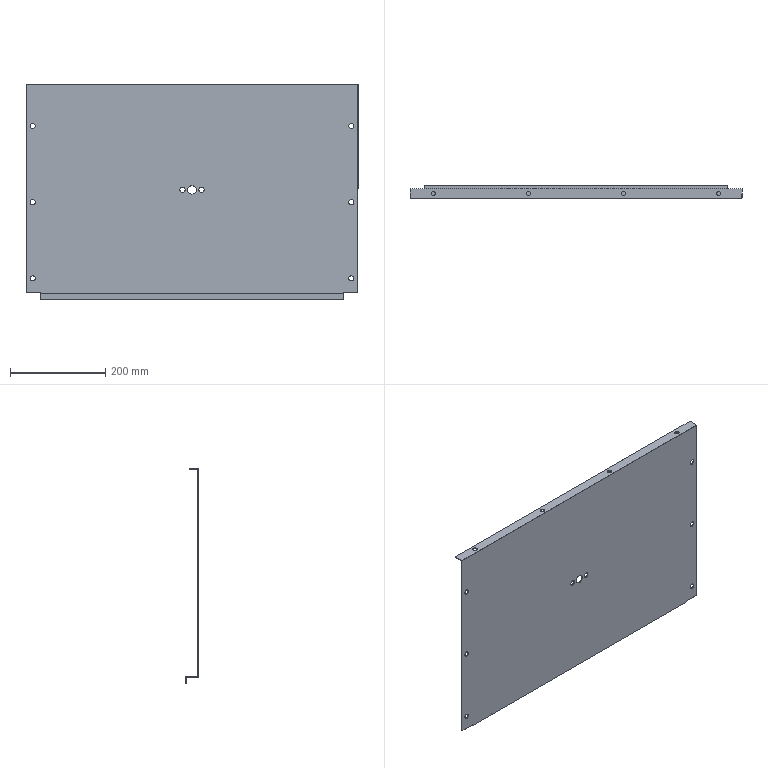Part | SolidWorks | features BaseBody 1 | 1 solid | 42 faces | box 698 x 28 x 453.25 mm | volume 686773 mm3 | cylinder 26 | plane 16 | commonest cylinder face diameters 10.6 x12 9.1 x8 11 x4 18 x2
STEP:
#1=CARTESIAN_POINT('',(211.946,-3643.973,1709.271));
#2=VERTEX_POINT('',#1);
#3=CARTESIAN_POINT('',(211.946,-3643.973,1698.671));
#4=VERTEX_POINT('',#3);
#5=CARTESIAN_POINT('',(211.946,-3643.973,1703.971));
#6=DIRECTION('',(0.,-1.,0.));
#7=DIRECTION('',(0.,0.,-1.));
#8=AXIS2_PLACEMENT_3D('',#5,#6,#7);
#9=CIRCLE('',#8,5.3);
#10=EDGE_CURVE('',#2,#4,#9,.T.);
#11=ORIENTED_EDGE('',*,*,#10,.F.);
#12=CARTESIAN_POINT('',(211.946,-3645.973,1709.271));
#13=VERTEX_POINT('',#12);
#14=CARTESIAN_POINT('',(211.946,-3631.556,1709.271));
#15=DIRECTION('',(0.,-1.,0.));
#16=VECTOR('',#15,1000.);
#17=LINE('',#14,#16);
#18=EDGE_CURVE('',#2,#13,#17,.T.);
#19=ORIENTED_EDGE('',*,*,#18,.T.);
#20=CARTESIAN_POINT('',(211.946,-3645.973,1698.671));
#21=VERTEX_POINT('',#20);
#22=CARTESIAN_POINT('',(211.946,-3645.973,1703.971));
#23=DIRECTION('',(0.,1.,0.));
#24=DIRECTION('',(0.,0.,-1.));
#25=AXIS2_PLACEMENT_3D('',#22,#23,#24);
#26=CIRCLE('',#25,5.3);
#27=EDGE_CURVE('',#21,#13,#26,.T.);
#28=ORIENTED_EDGE('',*,*,#27,.F.);
#29=CARTESIAN_POINT('',(211.946,-3631.556,1698.671));
#30=DIRECTION('',(0.,-1.,0.));
#31=VECTOR('',#30,1000.);
#32=LINE('',#29,#31);
#33=EDGE_CURVE('',#4,#21,#32,.T.);
#34=ORIENTED_EDGE('',*,*,#33,.F.);
#35=EDGE_LOOP('',(#11,#19,#28,#34));
#36=FACE_OUTER_BOUND('',#35,.T.);
#37=CARTESIAN_POINT('',(211.946,-3631.556,1703.971));
#38=DIRECTION('',(0.,-1.,0.));
#39=DIRECTION('',(0.,0.,-1.));
#40=AXIS2_PLACEMENT_3D('',#37,#38,#39);
#41=CYLINDRICAL_SURFACE('',#40,5.3);
#42=ADVANCED_FACE('',(#36),#41,.F.);
#43=CARTESIAN_POINT('',(211.946,-3643.973,2029.271));
#44=VERTEX_POINT('',#43);
#45=CARTESIAN_POINT('',(211.946,-3643.973,2018.671));
#46=VERTEX_POINT('',#45);
#47=CARTESIAN_POINT('',(211.946,-3643.973,2023.971));
#48=DIRECTION('',(0.,-1.,0.));
#49=DIRECTION('',(0.,0.,-1.));
#50=AXIS2_PLACEMENT_3D('',#47,#48,#49);
#51=CIRCLE('',#50,5.3);
#52=EDGE_CURVE('',#44,#46,#51,.T.);
#53=ORIENTED_EDGE('',*,*,#52,.F.);
#54=CARTESIAN_POINT('',(211.946,-3645.973,2029.271));
#55=VERTEX_POINT('',#54);
#56=CARTESIAN_POINT('',(211.946,-3631.556,2029.271));
#57=DIRECTION('',(0.,-1.,0.));
#58=VECTOR('',#57,1000.);
#59=LINE('',#56,#58);
#60=EDGE_CURVE('',#44,#55,#59,.T.);
#61=ORIENTED_EDGE('',*,*,#60,.T.);
#62=CARTESIAN_POINT('',(211.946,-3645.973,2018.671));
#63=VERTEX_POINT('',#62);
#64=CARTESIAN_POINT('',(211.946,-3645.973,2023.971));
#65=DIRECTION('',(0.,1.,0.));
#66=DIRECTION('',(0.,0.,-1.));
#67=AXIS2_PLACEMENT_3D('',#64,#65,#66);
#68=CIRCLE('',#67,5.3);
#69=EDGE_CURVE('',#63,#55,#68,.T.);
#70=ORIENTED_EDGE('',*,*,#69,.F.);
#71=CARTESIAN_POINT('',(211.946,-3631.556,2018.671));
#72=DIRECTION('',(0.,-1.,0.));
#73=VECTOR('',#72,1000.);
#74=LINE('',#71,#73);
#75=EDGE_CURVE('',#46,#63,#74,.T.);
#76=ORIENTED_EDGE('',*,*,#75,.F.);
#77=EDGE_LOOP('',(#53,#61,#70,#76));
#78=FACE_OUTER_BOUND('',#77,.T.);
#79=CARTESIAN_POINT('',(211.946,-3631.556,2023.971));
#80=DIRECTION('',(0.,-1.,0.));
#81=DIRECTION('',(0.,0.,-1.));
#82=AXIS2_PLACEMENT_3D('',#79,#80,#81);
#83=CYLINDRICAL_SURFACE('',#82,5.3);
#84=ADVANCED_FACE('',(#78),#83,.F.);
#85=CARTESIAN_POINT('',(881.946,-3645.973,1858.671));
#86=VERTEX_POINT('',#85);
#87=CARTESIAN_POINT('',(881.946,-3645.973,1869.271));
#88=VERTEX_POINT('',#87);
#89=CARTESIAN_POINT('',(881.946,-3645.973,1863.971));
#90=DIRECTION('',(0.,1.,0.));
#91=DIRECTION('',(0.,0.,1.));
#92=AXIS2_PLACEMENT_3D('',#89,#90,#91);
#93=CIRCLE('',#92,5.3);
#94=EDGE_CURVE('',#86,#88,#93,.T.);
#95=ORIENTED_EDGE('',*,*,#94,.F.);
#96=CARTESIAN_POINT('',(881.946,-3643.973,1858.671));
#97=VERTEX_POINT('',#96);
#98=CARTESIAN_POINT('',(881.946,-3631.556,1858.671));
#99=DIRECTION('',(0.,1.,0.));
#100=VECTOR('',#99,1000.);
#101=LINE('',#98,#100);
#102=EDGE_CURVE('',#86,#97,#101,.T.);
#103=ORIENTED_EDGE('',*,*,#102,.T.);
#104=CARTESIAN_POINT('',(881.946,-3643.973,1869.271));
#105=VERTEX_POINT('',#104);
#106=CARTESIAN_POINT('',(881.946,-3643.973,1863.971));
#107=DIRECTION('',(0.,-1.,0.));
#108=DIRECTION('',(0.,0.,1.));
#109=AXIS2_PLACEMENT_3D('',#106,#107,#108);
#110=CIRCLE('',#109,5.3);
#111=EDGE_CURVE('',#105,#97,#110,.T.);
#112=ORIENTED_EDGE('',*,*,#111,.F.);
#113=CARTESIAN_POINT('',(881.946,-3631.556,1869.271));
#114=DIRECTION('',(0.,1.,0.));
#115=VECTOR('',#114,1000.);
#116=LINE('',#113,#115);
#117=EDGE_CURVE('',#88,#105,#116,.T.);
#118=ORIENTED_EDGE('',*,*,#117,.F.);
#119=EDGE_LOOP('',(#95,#103,#112,#118));
#120=FACE_OUTER_BOUND('',#119,.T.);
#121=CARTESIAN_POINT('',(881.946,-3631.556,1863.971));
#122=DIRECTION('',(0.,1.,0.));
#123=DIRECTION('',(0.,0.,1.));
#124=AXIS2_PLACEMENT_3D('',#121,#122,#123);
#125=CYLINDRICAL_SURFACE('',#124,5.3);
#126=ADVANCED_FACE('',(#120),#125,.F.);
#127=CARTESIAN_POINT('',(881.946,-3645.973,2018.671));
#128=VERTEX_POINT('',#127);
#129=CARTESIAN_POINT('',(881.946,-3645.973,2029.271));
#130=VERTEX_POINT('',#129);
#131=CARTESIAN_POINT('',(881.946,-3645.973,2023.971));
#132=DIRECTION('',(0.,1.,0.));
#133=DIRECTION('',(0.,0.,1.));
#134=AXIS2_PLACEMENT_3D('',#131,#132,#133);
#135=CIRCLE('',#134,5.3);
#136=EDGE_CURVE('',#128,#130,#135,.T.);
#137=ORIENTED_EDGE('',*,*,#136,.F.);
#138=CARTESIAN_POINT('',(881.946,-3643.973,2018.671));
#139=VERTEX_POINT('',#138);
#140=CARTESIAN_POINT('',(881.946,-3631.556,2018.671));
#141=DIRECTION('',(0.,1.,0.));
#142=VECTOR('',#141,1000.);
#143=LINE('',#140,#142);
#144=EDGE_CURVE('',#128,#139,#143,.T.);
#145=ORIENTED_EDGE('',*,*,#144,.T.);
#146=CARTESIAN_POINT('',(881.946,-3643.973,2029.271));
#147=VERTEX_POINT('',#146);
#148=CARTESIAN_POINT('',(881.946,-3643.973,2023.971));
#149=DIRECTION('',(0.,-1.,0.));
#150=DIRECTION('',(0.,0.,1.));
#151=AXIS2_PLACEMENT_3D('',#148,#149,#150);
#152=CIRCLE('',#151,5.3);
#153=EDGE_CURVE('',#147,#139,#152,.T.);
#154=ORIENTED_EDGE('',*,*,#153,.F.);
#155=CARTESIAN_POINT('',(881.946,-3631.556,2029.271));
#156=DIRECTION('',(0.,1.,0.));
#157=VECTOR('',#156,1000.);
#158=LINE('',#155,#157);
#159=EDGE_CURVE('',#130,#147,#158,.T.);
#160=ORIENTED_EDGE('',*,*,#159,.F.);
#161=EDGE_LOOP('',(#137,#145,#154,#160));
#162=FACE_OUTER_BOUND('',#161,.T.);
#163=CARTESIAN_POINT('',(881.946,-3631.556,2023.971));
#164=DIRECTION('',(0.,1.,0.));
#165=DIRECTION('',(0.,0.,1.));
#166=AXIS2_PLACEMENT_3D('',#163,#164,#165);
#167=CYLINDRICAL_SURFACE('',#166,5.3);
#168=ADVANCED_FACE('',(#162),#167,.F.);
#169=CARTESIAN_POINT('',(881.946,-3645.973,1698.671));
#170=VERTEX_POINT('',#169);
#171=CARTESIAN_POINT('',(881.946,-3645.973,1709.271));
#172=VERTEX_POINT('',#171);
#173=CARTESIAN_POINT('',(881.946,-3645.973,1703.971));
#174=DIRECTION('',(0.,1.,0.));
#175=DIRECTION('',(0.,0.,1.));
#176=AXIS2_PLACEMENT_3D('',#173,#174,#175);
#177=CIRCLE('',#176,5.3);
#178=EDGE_CURVE('',#170,#172,#177,.T.);
#179=ORIENTED_EDGE('',*,*,#178,.F.);
#180=CARTESIAN_POINT('',(881.946,-3643.973,1698.671));
#181=VERTEX_POINT('',#180);
#182=CARTESIAN_POINT('',(881.946,-3631.556,1698.671));
#183=DIRECTION('',(0.,1.,0.));
#184=VECTOR('',#183,1000.);
#185=LINE('',#182,#184);
#186=EDGE_CURVE('',#170,#181,#185,.T.);
#187=ORIENTED_EDGE('',*,*,#186,.T.);
#188=CARTESIAN_POINT('',(881.946,-3643.973,1709.271));
#189=VERTEX_POINT('',#188);
#190=CARTESIAN_POINT('',(881.946,-3643.973,1703.971));
#191=DIRECTION('',(0.,-1.,0.));
#192=DIRECTION('',(0.,0.,1.));
#193=AXIS2_PLACEMENT_3D('',#190,#191,#192);
#194=CIRCLE('',#193,5.3);
#195=EDGE_CURVE('',#189,#181,#194,.T.);
#196=ORIENTED_EDGE('',*,*,#195,.F.);
#197=CARTESIAN_POINT('',(881.946,-3631.556,1709.271));
#198=DIRECTION('',(0.,1.,0.));
#199=VECTOR('',#198,1000.);
#200=LINE('',#197,#199);
#201=EDGE_CURVE('',#172,#189,#200,.T.);
#202=ORIENTED_EDGE('',*,*,#201,.F.);
#203=EDGE_LOOP('',(#179,#187,#196,#202));
#204=FACE_OUTER_BOUND('',#203,.T.);
#205=CARTESIAN_POINT('',(881.946,-3631.556,1703.971));
#206=DIRECTION('',(0.,1.,0.));
#207=DIRECTION('',(0.,0.,1.));
#208=AXIS2_PLACEMENT_3D('',#205,#206,#207);
#209=CYLINDRICAL_SURFACE('',#208,5.3);
#210=ADVANCED_FACE('',(#204),#209,.F.);
#211=CARTESIAN_POINT('',(211.946,-3643.973,1869.271));
#212=VERTEX_POINT('',#211);
#213=CARTESIAN_POINT('',(211.946,-3643.973,1858.671));
#214=VERTEX_POINT('',#213);
#215=CARTESIAN_POINT('',(211.946,-3643.973,1863.971));
#216=DIRECTION('',(0.,-1.,0.));
#217=DIRECTION('',(0.,0.,-1.));
#218=AXIS2_PLACEMENT_3D('',#215,#216,#217);
#219=CIRCLE('',#218,5.3);
#220=EDGE_CURVE('',#212,#214,#219,.T.);
#221=ORIENTED_EDGE('',*,*,#220,.F.);
#222=CARTESIAN_POINT('',(211.946,-3645.973,1869.271));
#223=VERTEX_POINT('',#222);
#224=CARTESIAN_POINT('',(211.946,-3631.556,1869.271));
#225=DIRECTION('',(0.,-1.,0.));
#226=VECTOR('',#225,1000.);
#227=LINE('',#224,#226);
#228=EDGE_CURVE('',#212,#223,#227,.T.);
#229=ORIENTED_EDGE('',*,*,#228,.T.);
#230=CARTESIAN_POINT('',(211.946,-3645.973,1858.671));
#231=VERTEX_POINT('',#230);
#232=CARTESIAN_POINT('',(211.946,-3645.973,1863.971));
#233=DIRECTION('',(0.,1.,0.));
#234=DIRECTION('',(0.,0.,-1.));
#235=AXIS2_PLACEMENT_3D('',#232,#233,#234);
#236=CIRCLE('',#235,5.3);
#237=EDGE_CURVE('',#231,#223,#236,.T.);
#238=ORIENTED_EDGE('',*,*,#237,.F.);
#239=CARTESIAN_POINT('',(211.946,-3631.556,1858.671));
#240=DIRECTION('',(0.,-1.,0.));
#241=VECTOR('',#240,1000.);
#242=LINE('',#239,#241);
#243=EDGE_CURVE('',#214,#231,#242,.T.);
#244=ORIENTED_EDGE('',*,*,#243,.F.);
#245=EDGE_LOOP('',(#221,#229,#238,#244));
#246=FACE_OUTER_BOUND('',#245,.T.);
#247=CARTESIAN_POINT('',(211.946,-3631.556,1863.971));
#248=DIRECTION('',(0.,-1.,0.));
#249=DIRECTION('',(0.,0.,-1.));
#250=AXIS2_PLACEMENT_3D('',#247,#248,#249);
#251=CYLINDRICAL_SURFACE('',#250,5.3);
#252=ADVANCED_FACE('',(#246),#251,.F.);
#253=CARTESIAN_POINT('',(526.946,-3643.973,1895.471));
#254=VERTEX_POINT('',#253);
#255=CARTESIAN_POINT('',(526.946,-3643.973,1884.471));
#256=VERTEX_POINT('',#255);
#257=CARTESIAN_POINT('',(526.946,-3643.973,1889.971));
#258=DIRECTION('',(0.,-1.,0.));
#259=DIRECTION('',(0.,0.,-1.));
#260=AXIS2_PLACEMENT_3D('',#257,#258,#259);
#261=CIRCLE('',#260,5.5);
#262=EDGE_CURVE('',#254,#256,#261,.T.);
#263=ORIENTED_EDGE('',*,*,#262,.F.);
#264=CARTESIAN_POINT('',(526.946,-3645.973,1895.471));
#265=VERTEX_POINT('',#264);
#266=CARTESIAN_POINT('',(526.946,-3653.934,1895.471));
#267=DIRECTION('',(0.,-1.,0.));
#268=VECTOR('',#267,1000.);
#269=LINE('',#266,#268);
#270=EDGE_CURVE('',#254,#265,#269,.T.);
#271=ORIENTED_EDGE('',*,*,#270,.T.);
#272=CARTESIAN_POINT('',(526.946,-3645.973,1884.471));
#273=VERTEX_POINT('',#272);
#274=CARTESIAN_POINT('',(526.946,-3645.973,1889.971));
#275=DIRECTION('',(0.,1.,0.));
#276=DIRECTION('',(0.,0.,-1.));
#277=AXIS2_PLACEMENT_3D('',#274,#275,#276);
#278=CIRCLE('',#277,5.5);
#279=EDGE_CURVE('',#273,#265,#278,.T.);
#280=ORIENTED_EDGE('',*,*,#279,.F.);
#281=CARTESIAN_POINT('',(526.946,-3653.934,1884.471));
#282=DIRECTION('',(0.,-1.,0.));
#283=VECTOR('',#282,1000.);
#284=LINE('',#281,#283);
#285=EDGE_CURVE('',#256,#273,#284,.T.);
#286=ORIENTED_EDGE('',*,*,#285,.F.);
#287=EDGE_LOOP('',(#263,#271,#280,#286));
#288=FACE_OUTER_BOUND('',#287,.T.);
#289=CARTESIAN_POINT('',(526.946,-3653.934,1889.971));
#290=DIRECTION('',(0.,-1.,0.));
#291=DIRECTION('',(0.,0.,-1.));
#292=AXIS2_PLACEMENT_3D('',#289,#290,#291);
#293=CYLINDRICAL_SURFACE('',#292,5.5);
#294=ADVANCED_FACE('',(#288),#293,.F.);
#295=CARTESIAN_POINT('',(566.946,-3645.973,1884.471));
#296=VERTEX_POINT('',#295);
#297=CARTESIAN_POINT('',(566.946,-3645.973,1895.471));
#298=VERTEX_POINT('',#297);
#299=CARTESIAN_POINT('',(566.946,-3645.973,1889.971));
#300=DIRECTION('',(0.,1.,0.));
#301=DIRECTION('',(0.,0.,1.));
#302=AXIS2_PLACEMENT_3D('',#299,#300,#301);
#303=CIRCLE('',#302,5.5);
#304=EDGE_CURVE('',#296,#298,#303,.T.);
#305=ORIENTED_EDGE('',*,*,#304,.F.);
#306=CARTESIAN_POINT('',(566.946,-3643.973,1884.471));
#307=VERTEX_POINT('',#306);
#308=CARTESIAN_POINT('',(566.946,-3653.934,1884.471));
#309=DIRECTION('',(0.,1.,0.));
#310=VECTOR('',#309,1000.);
#311=LINE('',#308,#310);
#312=EDGE_CURVE('',#296,#307,#311,.T.);
#313=ORIENTED_EDGE('',*,*,#312,.T.);
#314=CARTESIAN_POINT('',(566.946,-3643.973,1895.471));
#315=VERTEX_POINT('',#314);
#316=CARTESIAN_POINT('',(566.946,-3643.973,1889.971));
#317=DIRECTION('',(0.,-1.,0.));
#318=DIRECTION('',(0.,0.,1.));
#319=AXIS2_PLACEMENT_3D('',#316,#317,#318);
#320=CIRCLE('',#319,5.5);
#321=EDGE_CURVE('',#315,#307,#320,.T.);
#322=ORIENTED_EDGE('',*,*,#321,.F.);
#323=CARTESIAN_POINT('',(566.946,-3653.934,1895.471));
#324=DIRECTION('',(0.,1.,0.));
#325=VECTOR('',#324,1000.);
#326=LINE('',#323,#325);
#327=EDGE_CURVE('',#298,#315,#326,.T.);
#328=ORIENTED_EDGE('',*,*,#327,.F.);
#329=EDGE_LOOP('',(#305,#313,#322,#328));
#330=FACE_OUTER_BOUND('',#329,.T.);
#331=CARTESIAN_POINT('',(566.946,-3653.934,1889.971));
#332=DIRECTION('',(0.,1.,0.));
#333=DIRECTION('',(0.,0.,1.));
#334=AXIS2_PLACEMENT_3D('',#331,#332,#333);
#335=CYLINDRICAL_SURFACE('',#334,5.5);
#336=ADVANCED_FACE('',(#330),#335,.F.);
#337=CARTESIAN_POINT('',(546.946,-3643.973,1898.971));
#338=VERTEX_POINT('',#337);
#339=CARTESIAN_POINT('',(546.946,-3643.973,1880.971));
#340=VERTEX_POINT('',#339);
#341=CARTESIAN_POINT('',(546.946,-3643.973,1889.971));
#342=DIRECTION('',(0.,-1.,0.));
#343=DIRECTION('',(0.,0.,-1.));
#344=AXIS2_PLACEMENT_3D('',#341,#342,#343);
#345=CIRCLE('',#344,9.);
#346=EDGE_CURVE('',#338,#340,#345,.T.);
#347=ORIENTED_EDGE('',*,*,#346,.F.);
#348=CARTESIAN_POINT('',(546.946,-3645.973,1898.971));
#349=VERTEX_POINT('',#348);
#350=CARTESIAN_POINT('',(546.946,-3642.444,1898.971));
#351=DIRECTION('',(0.,-1.,0.));
#352=VECTOR('',#351,1000.);
#353=LINE('',#350,#352);
#354=EDGE_CURVE('',#338,#349,#353,.T.);
#355=ORIENTED_EDGE('',*,*,#354,.T.);
#356=CARTESIAN_POINT('',(546.946,-3645.973,1880.971));
#357=VERTEX_POINT('',#356);
#358=CARTESIAN_POINT('',(546.946,-3645.973,1889.971));
#359=DIRECTION('',(0.,1.,0.));
#360=DIRECTION('',(0.,0.,-1.));
#361=AXIS2_PLACEMENT_3D('',#358,#359,#360);
#362=CIRCLE('',#361,9.);
#363=EDGE_CURVE('',#357,#349,#362,.T.);
#364=ORIENTED_EDGE('',*,*,#363,.F.);
#365=CARTESIAN_POINT('',(546.946,-3642.444,1880.971));
#366=DIRECTION('',(0.,-1.,0.));
#367=VECTOR('',#366,1000.);
#368=LINE('',#365,#367);
#369=EDGE_CURVE('',#340,#357,#368,.T.);
#370=ORIENTED_EDGE('',*,*,#369,.F.);
#371=EDGE_LOOP('',(#347,#355,#364,#370));
#372=FACE_OUTER_BOUND('',#371,.T.);
#373=CARTESIAN_POINT('',(546.946,-3642.444,1889.971));
#374=DIRECTION('',(0.,-1.,0.));
#375=DIRECTION('',(0.,0.,-1.));
#376=AXIS2_PLACEMENT_3D('',#373,#374,#375);
#377=CYLINDRICAL_SURFACE('',#376,9.);
#378=ADVANCED_FACE('',(#372),#377,.F.);
#379=CARTESIAN_POINT('',(242.396,-3635.973,2109.971));
#380=VERTEX_POINT('',#379);
#381=CARTESIAN_POINT('',(251.496,-3635.973,2109.971));
#382=VERTEX_POINT('',#381);
#383=CARTESIAN_POINT('',(246.946,-3635.973,2109.971));
#384=DIRECTION('',(0.,0.,1.));
#385=DIRECTION('',(1.,0.,0.));
#386=AXIS2_PLACEMENT_3D('',#383,#384,#385);
#387=CIRCLE('',#386,4.55);
#388=EDGE_CURVE('',#380,#382,#387,.T.);
#389=ORIENTED_EDGE('',*,*,#388,.F.);
#390=CARTESIAN_POINT('',(242.396,-3635.973,2111.971));
#391=VERTEX_POINT('',#390);
#392=CARTESIAN_POINT('',(242.396,-3635.973,2133.845));
#393=DIRECTION('',(0.,0.,1.));
#394=VECTOR('',#393,1000.);
#395=LINE('',#392,#394);
#396=EDGE_CURVE('',#380,#391,#395,.T.);
#397=ORIENTED_EDGE('',*,*,#396,.T.);
#398=CARTESIAN_POINT('',(251.496,-3635.973,2111.971));
#399=VERTEX_POINT('',#398);
#400=CARTESIAN_POINT('',(246.946,-3635.973,2111.971));
#401=DIRECTION('',(0.,0.,-1.));
#402=DIRECTION('',(1.,0.,0.));
#403=AXIS2_PLACEMENT_3D('',#400,#401,#402);
#404=CIRCLE('',#403,4.55);
#405=EDGE_CURVE('',#399,#391,#404,.T.);
#406=ORIENTED_EDGE('',*,*,#405,.F.);
#407=CARTESIAN_POINT('',(251.496,-3635.973,2133.845));
#408=DIRECTION('',(0.,0.,1.));
#409=VECTOR('',#408,1000.);
#410=LINE('',#407,#409);
#411=EDGE_CURVE('',#382,#399,#410,.T.);
#412=ORIENTED_EDGE('',*,*,#411,.F.);
#413=EDGE_LOOP('',(#389,#397,#406,#412));
#414=FACE_OUTER_BOUND('',#413,.T.);
#415=CARTESIAN_POINT('',(246.946,-3635.973,2133.845));
#416=DIRECTION('',(0.,0.,1.));
#417=DIRECTION('',(1.,0.,0.));
#418=AXIS2_PLACEMENT_3D('',#415,#416,#417);
#419=CYLINDRICAL_SURFACE('',#418,4.55);
#420=ADVANCED_FACE('',(#414),#419,.F.);
#421=CARTESIAN_POINT('',(851.496,-3635.973,2111.971));
#422=VERTEX_POINT('',#421);
#423=CARTESIAN_POINT('',(842.396,-3635.973,2111.971));
#424=VERTEX_POINT('',#423);
#425=CARTESIAN_POINT('',(846.946,-3635.973,2111.971));
#426=DIRECTION('',(0.,0.,-1.));
#427=DIRECTION('',(-1.,0.,0.));
#428=AXIS2_PLACEMENT_3D('',#425,#426,#427);
#429=CIRCLE('',#428,4.55);
#430=EDGE_CURVE('',#422,#424,#429,.T.);
#431=ORIENTED_EDGE('',*,*,#430,.F.);
#432=CARTESIAN_POINT('',(851.496,-3635.973,2109.971));
#433=VERTEX_POINT('',#432);
#434=CARTESIAN_POINT('',(851.496,-3635.973,2133.845));
#435=DIRECTION('',(0.,0.,-1.));
#436=VECTOR('',#435,1000.);
#437=LINE('',#434,#436);
#438=EDGE_CURVE('',#422,#433,#437,.T.);
#439=ORIENTED_EDGE('',*,*,#438,.T.);
#440=CARTESIAN_POINT('',(842.396,-3635.973,2109.971));
#441=VERTEX_POINT('',#440);
#442=CARTESIAN_POINT('',(846.946,-3635.973,2109.971));
#443=DIRECTION('',(0.,0.,1.));
#444=DIRECTION('',(-1.,0.,0.));
#445=AXIS2_PLACEMENT_3D('',#442,#443,#444);
#446=CIRCLE('',#445,4.55);
#447=EDGE_CURVE('',#441,#433,#446,.T.);
#448=ORIENTED_EDGE('',*,*,#447,.F.);
#449=CARTESIAN_POINT('',(842.396,-3635.973,2133.845));
#450=DIRECTION('',(0.,0.,-1.));
#451=VECTOR('',#450,1000.);
#452=LINE('',#449,#451);
#453=EDGE_CURVE('',#424,#441,#452,.T.);
#454=ORIENTED_EDGE('',*,*,#453,.F.);
#455=EDGE_LOOP('',(#431,#439,#448,#454));
#456=FACE_OUTER_BOUND('',#455,.T.);
#457=CARTESIAN_POINT('',(846.946,-3635.973,2133.845));
#458=DIRECTION('',(0.,0.,-1.));
#459=DIRECTION('',(-1.,0.,0.));
#460=AXIS2_PLACEMENT_3D('',#457,#458,#459);
#461=CYLINDRICAL_SURFACE('',#460,4.55);
#462=ADVANCED_FACE('',(#456),#461,.F.);
#463=CARTESIAN_POINT('',(651.496,-3635.973,2111.971));
#464=VERTEX_POINT('',#463);
#465=CARTESIAN_POINT('',(642.396,-3635.973,2111.971));
#466=VERTEX_POINT('',#465);
#467=CARTESIAN_POINT('',(646.946,-3635.973,2111.971));
#468=DIRECTION('',(0.,0.,-1.));
#469=DIRECTION('',(-1.,0.,0.));
#470=AXIS2_PLACEMENT_3D('',#467,#468,#469);
#471=CIRCLE('',#470,4.55);
#472=EDGE_CURVE('',#464,#466,#471,.T.);
#473=ORIENTED_EDGE('',*,*,#472,.F.);
#474=CARTESIAN_POINT('',(651.496,-3635.973,2109.971));
#475=VERTEX_POINT('',#474);
#476=CARTESIAN_POINT('',(651.496,-3635.973,2133.845));
#477=DIRECTION('',(0.,0.,-1.));
#478=VECTOR('',#477,1000.);
#479=LINE('',#476,#478);
#480=EDGE_CURVE('',#464,#475,#479,.T.);
#481=ORIENTED_EDGE('',*,*,#480,.T.);
#482=CARTESIAN_POINT('',(642.396,-3635.973,2109.971));
#483=VERTEX_POINT('',#482);
#484=CARTESIAN_POINT('',(646.946,-3635.973,2109.971));
#485=DIRECTION('',(0.,0.,1.));
#486=DIRECTION('',(-1.,0.,0.));
#487=AXIS2_PLACEMENT_3D('',#484,#485,#486);
#488=CIRCLE('',#487,4.55);
#489=EDGE_CURVE('',#483,#475,#488,.T.);
#490=ORIENTED_EDGE('',*,*,#489,.F.);
#491=CARTESIAN_POINT('',(642.396,-3635.973,2133.845));
#492=DIRECTION('',(0.,0.,-1.));
#493=VECTOR('',#492,1000.);
#494=LINE('',#491,#493);
#495=EDGE_CURVE('',#466,#483,#494,.T.);
#496=ORIENTED_EDGE('',*,*,#495,.F.);
#497=EDGE_LOOP('',(#473,#481,#490,#496));
#498=FACE_OUTER_BOUND('',#497,.T.);
#499=CARTESIAN_POINT('',(646.946,-3635.973,2133.845));
#500=DIRECTION('',(0.,0.,-1.));
#501=DIRECTION('',(-1.,0.,0.));
#502=AXIS2_PLACEMENT_3D('',#499,#500,#501);
#503=CYLINDRICAL_SURFACE('',#502,4.55);
#504=ADVANCED_FACE('',(#498),#503,.F.);
#505=CARTESIAN_POINT('',(442.396,-3635.973,2109.971));
#506=VERTEX_POINT('',#505);
#507=CARTESIAN_POINT('',(451.496,-3635.973,2109.971));
#508=VERTEX_POINT('',#507);
#509=CARTESIAN_POINT('',(446.946,-3635.973,2109.971));
#510=DIRECTION('',(0.,0.,1.));
#511=DIRECTION('',(1.,0.,0.));
#512=AXIS2_PLACEMENT_3D('',#509,#510,#511);
#513=CIRCLE('',#512,4.55);
#514=EDGE_CURVE('',#506,#508,#513,.T.);
#515=ORIENTED_EDGE('',*,*,#514,.F.);
#516=CARTESIAN_POINT('',(442.396,-3635.973,2111.971));
#517=VERTEX_POINT('',#516);
#518=CARTESIAN_POINT('',(442.396,-3635.973,2133.845));
#519=DIRECTION('',(0.,0.,1.));
#520=VECTOR('',#519,1000.);
#521=LINE('',#518,#520);
#522=EDGE_CURVE('',#506,#517,#521,.T.);
#523=ORIENTED_EDGE('',*,*,#522,.T.);
#524=CARTESIAN_POINT('',(451.496,-3635.973,2111.971));
#525=VERTEX_POINT('',#524);
#526=CARTESIAN_POINT('',(446.946,-3635.973,2111.971));
#527=DIRECTION('',(0.,0.,-1.));
#528=DIRECTION('',(1.,0.,0.));
#529=AXIS2_PLACEMENT_3D('',#526,#527,#528);
#530=CIRCLE('',#529,4.55);
#531=EDGE_CURVE('',#525,#517,#530,.T.);
#532=ORIENTED_EDGE('',*,*,#531,.F.);
#533=CARTESIAN_POINT('',(451.496,-3635.973,2133.845));
#534=DIRECTION('',(0.,0.,1.));
#535=VECTOR('',#534,1000.);
#536=LINE('',#533,#535);
#537=EDGE_CURVE('',#508,#525,#536,.T.);
#538=ORIENTED_EDGE('',*,*,#537,.F.);
#539=EDGE_LOOP('',(#515,#523,#532,#538));
#540=FACE_OUTER_BOUND('',#539,.T.);
#541=CARTESIAN_POINT('',(446.946,-3635.973,2133.845));
#542=DIRECTION('',(0.,0.,1.));
#543=DIRECTION('',(1.,0.,0.));
#544=AXIS2_PLACEMENT_3D('',#541,#542,#543);
#545=CYLINDRICAL_SURFACE('',#544,4.55);
#546=ADVANCED_FACE('',(#540),#545,.F.);
#547=CARTESIAN_POINT('',(895.946,-3645.973,1673.721));
#548=VERTEX_POINT('',#547);
#549=CARTESIAN_POINT('',(895.946,-3645.973,2111.971));
#550=VERTEX_POINT('',#549);
#551=CARTESIAN_POINT('',(895.946,-3645.973,2111.971));
#552=DIRECTION('',(0.,0.,1.));
#553=VECTOR('',#552,1000.);
#554=LINE('',#551,#553);
#555=EDGE_CURVE('',#548,#550,#554,.T.);
#556=ORIENTED_EDGE('',*,*,#555,.T.);
#557=CARTESIAN_POINT('',(197.946,-3645.973,2111.971));
#558=VERTEX_POINT('',#557);
#559=CARTESIAN_POINT('',(895.946,-3645.973,2111.971));
#560=DIRECTION('',(-1.,0.,0.));
#561=VECTOR('',#560,1000.);
#562=LINE('',#559,#561);
#563=EDGE_CURVE('',#550,#558,#562,.T.);
#564=ORIENTED_EDGE('',*,*,#563,.T.);
#565=CARTESIAN_POINT('',(197.946,-3645.973,1673.721));
#566=VERTEX_POINT('',#565);
#567=CARTESIAN_POINT('',(197.946,-3645.973,2111.971));
#568=DIRECTION('',(0.,0.,-1.));
#569=VECTOR('',#568,1000.);
#570=LINE('',#567,#569);
#571=EDGE_CURVE('',#558,#566,#570,.T.);
#572=ORIENTED_EDGE('',*,*,#571,.T.);
#573=CARTESIAN_POINT('',(227.946,-3645.973,1673.721));
#574=VERTEX_POINT('',#573);
#575=CARTESIAN_POINT('',(895.946,-3645.973,1673.721));
#576=DIRECTION('',(1.,0.,0.));
#577=VECTOR('',#576,1000.);
#578=LINE('',#575,#577);
#579=EDGE_CURVE('',#566,#574,#578,.T.);
#580=ORIENTED_EDGE('',*,*,#579,.T.);
#581=CARTESIAN_POINT('',(227.946,-3645.973,1671.721));
#582=VERTEX_POINT('',#581);
#583=CARTESIAN_POINT('',(227.946,-3645.973,2111.971));
#584=DIRECTION('',(0.,0.,-1.));
#585=VECTOR('',#584,1000.);
#586=LINE('',#583,#585);
#587=EDGE_CURVE('',#574,#582,#586,.T.);
#588=ORIENTED_EDGE('',*,*,#587,.T.);
#589=CARTESIAN_POINT('',(865.946,-3645.973,1671.721));
#590=VERTEX_POINT('',#589);
#591=CARTESIAN_POINT('',(895.946,-3645.973,1671.721));
#592=DIRECTION('',(1.,0.,0.));
#593=VECTOR('',#592,1000.);
#594=LINE('',#591,#593);
#595=EDGE_CURVE('',#582,#590,#594,.T.);
#596=ORIENTED_EDGE('',*,*,#595,.T.);
#597=CARTESIAN_POINT('',(865.946,-3645.973,1673.721));
#598=VERTEX_POINT('',#597);
#599=CARTESIAN_POINT('',(865.946,-3645.973,2111.971));
#600=DIRECTION('',(0.,0.,1.));
#601=VECTOR('',#600,1000.);
#602=LINE('',#599,#601);
#603=EDGE_CURVE('',#590,#598,#602,.T.);
#604=ORIENTED_EDGE('',*,*,#603,.T.);
#605=CARTESIAN_POINT('',(895.946,-3645.973,1673.721));
#606=DIRECTION('',(1.,0.,0.));
#607=VECTOR('',#606,1000.);
#608=LINE('',#605,#607);
#609=EDGE_CURVE('',#598,#548,#608,.T.);
#610=ORIENTED_EDGE('',*,*,#609,.T.);
#611=EDGE_LOOP('',(#556,#564,#572,#580,#588,#596,#604,#610));
#612=FACE_OUTER_BOUND('',#611,.T.);
#613=ORIENTED_EDGE('',*,*,#27,.T.);
#614=CARTESIAN_POINT('',(211.946,-3645.973,1703.971));
#615=DIRECTION('',(0.,1.,0.));
#616=DIRECTION('',(0.,0.,-1.));
#617=AXIS2_PLACEMENT_3D('',#614,#615,#616);
#618=CIRCLE('',#617,5.3);
#619=EDGE_CURVE('',#13,#21,#618,.T.);
#620=ORIENTED_EDGE('',*,*,#619,.T.);
#621=EDGE_LOOP('',(#613,#620));
#622=FACE_BOUND('',#621,.T.);
#623=ORIENTED_EDGE('',*,*,#69,.T.);
#624=CARTESIAN_POINT('',(211.946,-3645.973,2023.971));
#625=DIRECTION('',(0.,1.,0.));
#626=DIRECTION('',(0.,0.,-1.));
#627=AXIS2_PLACEMENT_3D('',#624,#625,#626);
#628=CIRCLE('',#627,5.3);
#629=EDGE_CURVE('',#55,#63,#628,.T.);
#630=ORIENTED_EDGE('',*,*,#629,.T.);
#631=EDGE_LOOP('',(#623,#630));
#632=FACE_BOUND('',#631,.T.);
#633=CARTESIAN_POINT('',(881.946,-3645.973,1863.971));
#634=DIRECTION('',(0.,1.,0.));
#635=DIRECTION('',(0.,0.,1.));
#636=AXIS2_PLACEMENT_3D('',#633,#634,#635);
#637=CIRCLE('',#636,5.3);
#638=EDGE_CURVE('',#88,#86,#637,.T.);
#639=ORIENTED_EDGE('',*,*,#638,.T.);
#640=ORIENTED_EDGE('',*,*,#94,.T.);
#641=EDGE_LOOP('',(#639,#640));
#642=FACE_BOUND('',#641,.T.);
#643=CARTESIAN_POINT('',(881.946,-3645.973,2023.971));
#644=DIRECTION('',(0.,1.,0.));
#645=DIRECTION('',(0.,0.,1.));
#646=AXIS2_PLACEMENT_3D('',#643,#644,#645);
#647=CIRCLE('',#646,5.3);
#648=EDGE_CURVE('',#130,#128,#647,.T.);
#649=ORIENTED_EDGE('',*,*,#648,.T.);
#650=ORIENTED_EDGE('',*,*,#136,.T.);
#651=EDGE_LOOP('',(#649,#650));
#652=FACE_BOUND('',#651,.T.);
#653=CARTESIAN_POINT('',(881.946,-3645.973,1703.971));
#654=DIRECTION('',(0.,1.,0.));
#655=DIRECTION('',(0.,0.,1.));
#656=AXIS2_PLACEMENT_3D('',#653,#654,#655);
#657=CIRCLE('',#656,5.3);
#658=EDGE_CURVE('',#172,#170,#657,.T.);
#659=ORIENTED_EDGE('',*,*,#658,.T.);
#660=ORIENTED_EDGE('',*,*,#178,.T.);
#661=EDGE_LOOP('',(#659,#660));
#662=FACE_BOUND('',#661,.T.);
#663=ORIENTED_EDGE('',*,*,#237,.T.);
#664=CARTESIAN_POINT('',(211.946,-3645.973,1863.971));
#665=DIRECTION('',(0.,1.,0.));
#666=DIRECTION('',(0.,0.,-1.));
#667=AXIS2_PLACEMENT_3D('',#664,#665,#666);
#668=CIRCLE('',#667,5.3);
#669=EDGE_CURVE('',#223,#231,#668,.T.);
#670=ORIENTED_EDGE('',*,*,#669,.T.);
#671=EDGE_LOOP('',(#663,#670));
#672=FACE_BOUND('',#671,.T.);
#673=ORIENTED_EDGE('',*,*,#279,.T.);
#674=CARTESIAN_POINT('',(526.946,-3645.973,1889.971));
#675=DIRECTION('',(0.,1.,0.));
#676=DIRECTION('',(0.,0.,-1.));
#677=AXIS2_PLACEMENT_3D('',#674,#675,#676);
#678=CIRCLE('',#677,5.5);
#679=EDGE_CURVE('',#265,#273,#678,.T.);
#680=ORIENTED_EDGE('',*,*,#679,.T.);
#681=EDGE_LOOP('',(#673,#680));
#682=FACE_BOUND('',#681,.T.);
#683=CARTESIAN_POINT('',(566.946,-3645.973,1889.971));
#684=DIRECTION('',(0.,1.,0.));
#685=DIRECTION('',(0.,0.,1.));
#686=AXIS2_PLACEMENT_3D('',#683,#684,#685);
#687=CIRCLE('',#686,5.5);
#688=EDGE_CURVE('',#298,#296,#687,.T.);
#689=ORIENTED_EDGE('',*,*,#688,.T.);
#690=ORIENTED_EDGE('',*,*,#304,.T.);
#691=EDGE_LOOP('',(#689,#690));
#692=FACE_BOUND('',#691,.T.);
#693=ORIENTED_EDGE('',*,*,#363,.T.);
#694=CARTESIAN_POINT('',(546.946,-3645.973,1889.971));
#695=DIRECTION('',(0.,1.,0.));
#696=DIRECTION('',(0.,0.,-1.));
#697=AXIS2_PLACEMENT_3D('',#694,#695,#696);
#698=CIRCLE('',#697,9.);
#699=EDGE_CURVE('',#349,#357,#698,.T.);
#700=ORIENTED_EDGE('',*,*,#699,.T.);
#701=EDGE_LOOP('',(#693,#700));
#702=FACE_BOUND('',#701,.T.);
#703=CARTESIAN_POINT('',(895.946,-3645.973,2111.971));
#704=DIRECTION('',(0.,-1.,0.));
#705=DIRECTION('',(0.,0.,-1.));
#706=AXIS2_PLACEMENT_3D('',#703,#704,#705);
#707=PLANE('',#706);
#708=ADVANCED_FACE('',(#612,#622,#632,#642,#652,#662,#672,#682,#692,#702),#707,.T.);
#709=ORIENTED_EDGE('',*,*,#405,.T.);
#710=CARTESIAN_POINT('',(246.946,-3635.973,2111.971));
#711=DIRECTION('',(0.,0.,-1.));
#712=DIRECTION('',(1.,0.,0.));
#713=AXIS2_PLACEMENT_3D('',#710,#711,#712);
#714=CIRCLE('',#713,4.55);
#715=EDGE_CURVE('',#391,#399,#714,.T.);
#716=ORIENTED_EDGE('',*,*,#715,.T.);
#717=EDGE_LOOP('',(#709,#716));
#718=FACE_BOUND('',#717,.T.);
#719=CARTESIAN_POINT('',(846.946,-3635.973,2111.971));
#720=DIRECTION('',(0.,0.,-1.));
#721=DIRECTION('',(-1.,0.,0.));
#722=AXIS2_PLACEMENT_3D('',#719,#720,#721);
#723=CIRCLE('',#722,4.55);
#724=EDGE_CURVE('',#424,#422,#723,.T.);
#725=ORIENTED_EDGE('',*,*,#724,.T.);
#726=ORIENTED_EDGE('',*,*,#430,.T.);
#727=EDGE_LOOP('',(#725,#726));
#728=FACE_BOUND('',#727,.T.);
#729=CARTESIAN_POINT('',(646.946,-3635.973,2111.971));
#730=DIRECTION('',(0.,0.,-1.));
#731=DIRECTION('',(-1.,0.,0.));
#732=AXIS2_PLACEMENT_3D('',#729,#730,#731);
#733=CIRCLE('',#732,4.55);
#734=EDGE_CURVE('',#466,#464,#733,.T.);
#735=ORIENTED_EDGE('',*,*,#734,.T.);
#736=ORIENTED_EDGE('',*,*,#472,.T.);
#737=EDGE_LOOP('',(#735,#736));
#738=FACE_BOUND('',#737,.T.);
#739=ORIENTED_EDGE('',*,*,#531,.T.);
#740=CARTESIAN_POINT('',(446.946,-3635.973,2111.971));
#741=DIRECTION('',(0.,0.,-1.));
#742=DIRECTION('',(1.,0.,0.));
#743=AXIS2_PLACEMENT_3D('',#740,#741,#742);
#744=CIRCLE('',#743,4.55);
#745=EDGE_CURVE('',#517,#525,#744,.T.);
#746=ORIENTED_EDGE('',*,*,#745,.T.);
#747=EDGE_LOOP('',(#739,#746));
#748=FACE_BOUND('',#747,.T.);
#749=CARTESIAN_POINT('',(197.946,-3625.973,2111.971));
#750=VERTEX_POINT('',#749);
#751=CARTESIAN_POINT('',(197.946,-3625.973,2111.971));
#752=DIRECTION('',(0.,-1.,0.));
#753=VECTOR('',#752,1000.);
#754=LINE('',#751,#753);
#755=EDGE_CURVE('',#750,#558,#754,.T.);
#756=ORIENTED_EDGE('',*,*,#755,.T.);
#757=ORIENTED_EDGE('',*,*,#563,.F.);
#758=CARTESIAN_POINT('',(895.946,-3625.973,2111.971));
#759=VERTEX_POINT('',#758);
#760=CARTESIAN_POINT('',(895.946,-3625.973,2111.971));
#761=DIRECTION('',(0.,1.,0.));
#762=VECTOR('',#761,1000.);
#763=LINE('',#760,#762);
#764=EDGE_CURVE('',#550,#759,#763,.T.);
#765=ORIENTED_EDGE('',*,*,#764,.T.);
#766=CARTESIAN_POINT('',(895.946,-3625.973,2111.971));
#767=DIRECTION('',(-1.,0.,0.));
#768=VECTOR('',#767,1000.);
#769=LINE('',#766,#768);
#770=EDGE_CURVE('',#759,#750,#769,.T.);
#771=ORIENTED_EDGE('',*,*,#770,.T.);
#772=EDGE_LOOP('',(#756,#757,#765,#771));
#773=FACE_OUTER_BOUND('',#772,.T.);
#774=CARTESIAN_POINT('',(895.946,-3625.973,2111.971));
#775=DIRECTION('',(0.,0.,1.));
#776=DIRECTION('',(1.,0.,0.));
#777=AXIS2_PLACEMENT_3D('',#774,#775,#776);
#778=PLANE('',#777);
#779=ADVANCED_FACE('',(#718,#728,#738,#748,#773),#778,.T.);
#780=CARTESIAN_POINT('',(895.946,-3643.973,1673.721));
#781=VERTEX_POINT('',#780);
#782=CARTESIAN_POINT('',(895.946,-3633.473,1673.721));
#783=DIRECTION('',(0.,1.,0.));
#784=VECTOR('',#783,1000.);
#785=LINE('',#782,#784);
#786=EDGE_CURVE('',#548,#781,#785,.T.);
#787=ORIENTED_EDGE('',*,*,#786,.T.);
#788=CARTESIAN_POINT('',(895.946,-3643.973,2109.971));
#789=VERTEX_POINT('',#788);
#790=CARTESIAN_POINT('',(895.946,-3643.973,2110.971));
#791=DIRECTION('',(0.,0.,1.));
#792=VECTOR('',#791,1000.);
#793=LINE('',#790,#792);
#794=EDGE_CURVE('',#781,#789,#793,.T.);
#795=ORIENTED_EDGE('',*,*,#794,.T.);
#796=CARTESIAN_POINT('',(895.946,-3625.973,2109.971));
#797=VERTEX_POINT('',#796);
#798=CARTESIAN_POINT('',(895.946,-3633.473,2109.971));
#799=DIRECTION('',(0.,1.,0.));
#800=VECTOR('',#799,1000.);
#801=LINE('',#798,#800);
#802=EDGE_CURVE('',#789,#797,#801,.T.);
#803=ORIENTED_EDGE('',*,*,#802,.T.);
#804=CARTESIAN_POINT('',(895.946,-3625.973,2110.971));
#805=DIRECTION('',(0.,0.,1.));
#806=VECTOR('',#805,1000.);
#807=LINE('',#804,#806);
#808=EDGE_CURVE('',#797,#759,#807,.T.);
#809=ORIENTED_EDGE('',*,*,#808,.T.);
#810=ORIENTED_EDGE('',*,*,#764,.F.);
#811=ORIENTED_EDGE('',*,*,#555,.F.);
#812=EDGE_LOOP('',(#787,#795,#803,#809,#810,#811));
#813=FACE_OUTER_BOUND('',#812,.T.);
#814=CARTESIAN_POINT('',(895.946,-3633.473,2110.971));
#815=DIRECTION('',(1.,0.,0.));
#816=DIRECTION('',(0.,0.,-1.));
#817=AXIS2_PLACEMENT_3D('',#814,#815,#816);
#818=PLANE('',#817);
#819=ADVANCED_FACE('',(#813),#818,.T.);
#820=CARTESIAN_POINT('',(865.946,-3643.973,1673.721));
#821=VERTEX_POINT('',#820);
#822=CARTESIAN_POINT('',(865.946,-3572.676,1673.721));
#823=DIRECTION('',(0.,-1.,0.));
#824=VECTOR('',#823,1000.);
#825=LINE('',#822,#824);
#826=EDGE_CURVE('',#821,#598,#825,.T.);
#827=ORIENTED_EDGE('',*,*,#826,.F.);
#828=CARTESIAN_POINT('',(945.946,-3643.973,1673.721));
#829=DIRECTION('',(-1.,0.,0.));
#830=VECTOR('',#829,1000.);
#831=LINE('',#828,#830);
#832=EDGE_CURVE('',#781,#821,#831,.T.);
#833=ORIENTED_EDGE('',*,*,#832,.F.);
#834=ORIENTED_EDGE('',*,*,#786,.F.);
#835=ORIENTED_EDGE('',*,*,#609,.F.);
#836=EDGE_LOOP('',(#827,#833,#834,#835));
#837=FACE_OUTER_BOUND('',#836,.T.);
#838=CARTESIAN_POINT('',(945.946,-3572.676,1673.721));
#839=DIRECTION('',(0.,0.,1.));
#840=DIRECTION('',(1.,0.,0.));
#841=AXIS2_PLACEMENT_3D('',#838,#839,#840);
#842=PLANE('',#841);
#843=ADVANCED_FACE('',(#837),#842,.F.);
#844=CARTESIAN_POINT('',(865.946,-3619.973,1671.721));
#845=VERTEX_POINT('',#844);
#846=CARTESIAN_POINT('',(865.946,-3578.676,1671.721));
#847=DIRECTION('',(0.,-1.,0.));
#848=VECTOR('',#847,1000.);
#849=LINE('',#846,#848);
#850=EDGE_CURVE('',#845,#590,#849,.T.);
#851=ORIENTED_EDGE('',*,*,#850,.F.);
#852=CARTESIAN_POINT('',(865.946,-3619.973,1658.721));
#853=VERTEX_POINT('',#852);
#854=CARTESIAN_POINT('',(865.946,-3619.973,1673.721));
#855=DIRECTION('',(0.,0.,1.));
#856=VECTOR('',#855,1000.);
#857=LINE('',#854,#856);
#858=EDGE_CURVE('',#853,#845,#857,.T.);
#859=ORIENTED_EDGE('',*,*,#858,.F.);
#860=CARTESIAN_POINT('',(865.946,-3617.973,1658.721));
#861=VERTEX_POINT('',#860);
#862=CARTESIAN_POINT('',(865.946,-3578.676,1658.721));
#863=DIRECTION('',(0.,-1.,0.));
#864=VECTOR('',#863,1000.);
#865=LINE('',#862,#864);
#866=EDGE_CURVE('',#861,#853,#865,.T.);
#867=ORIENTED_EDGE('',*,*,#866,.F.);
#868=CARTESIAN_POINT('',(865.946,-3617.973,1673.721));
#869=VERTEX_POINT('',#868);
#870=CARTESIAN_POINT('',(865.946,-3617.973,1673.721));
#871=DIRECTION('',(0.,0.,-1.));
#872=VECTOR('',#871,1000.);
#873=LINE('',#870,#872);
#874=EDGE_CURVE('',#869,#861,#873,.T.);
#875=ORIENTED_EDGE('',*,*,#874,.F.);
#876=CARTESIAN_POINT('',(865.946,-3578.676,1673.721));
#877=DIRECTION('',(0.,1.,0.));
#878=VECTOR('',#877,1000.);
#879=LINE('',#876,#878);
#880=EDGE_CURVE('',#821,#869,#879,.T.);
#881=ORIENTED_EDGE('',*,*,#880,.F.);
#882=ORIENTED_EDGE('',*,*,#826,.T.);
#883=ORIENTED_EDGE('',*,*,#603,.F.);
#884=EDGE_LOOP('',(#851,#859,#867,#875,#881,#882,#883));
#885=FACE_OUTER_BOUND('',#884,.T.);
#886=CARTESIAN_POINT('',(865.946,-3578.676,1673.721));
#887=DIRECTION('',(-1.,0.,0.));
#888=DIRECTION('',(0.,0.,1.));
#889=AXIS2_PLACEMENT_3D('',#886,#887,#888);
#890=PLANE('',#889);
#891=ADVANCED_FACE('',(#885),#890,.F.);
#892=ORIENTED_EDGE('',*,*,#850,.T.);
#893=ORIENTED_EDGE('',*,*,#595,.F.);
#894=CARTESIAN_POINT('',(227.946,-3619.973,1671.721));
#895=VERTEX_POINT('',#894);
#896=CARTESIAN_POINT('',(227.946,-3645.973,1671.721));
#897=DIRECTION('',(0.,1.,0.));
#898=VECTOR('',#897,1000.);
#899=LINE('',#896,#898);
#900=EDGE_CURVE('',#582,#895,#899,.T.);
#901=ORIENTED_EDGE('',*,*,#900,.T.);
#902=CARTESIAN_POINT('',(926.946,-3619.973,1671.721));
#903=DIRECTION('',(1.,0.,0.));
#904=VECTOR('',#903,1000.);
#905=LINE('',#902,#904);
#906=EDGE_CURVE('',#895,#845,#905,.T.);
#907=ORIENTED_EDGE('',*,*,#906,.T.);
#908=EDGE_LOOP('',(#892,#893,#901,#907));
#909=FACE_OUTER_BOUND('',#908,.T.);
#910=CARTESIAN_POINT('',(926.946,-3645.973,1671.721));
#911=DIRECTION('',(0.,0.,-1.));
#912=DIRECTION('',(-1.,0.,0.));
#913=AXIS2_PLACEMENT_3D('',#910,#911,#912);
#914=PLANE('',#913);
#915=ADVANCED_FACE('',(#909),#914,.T.);
#916=CARTESIAN_POINT('',(227.946,-3643.973,1673.721));
#917=VERTEX_POINT('',#916);
#918=CARTESIAN_POINT('',(227.946,-3566.676,1673.721));
#919=DIRECTION('',(0.,-1.,0.));
#920=VECTOR('',#919,1000.);
#921=LINE('',#918,#920);
#922=EDGE_CURVE('',#917,#574,#921,.T.);
#923=ORIENTED_EDGE('',*,*,#922,.F.);
#924=CARTESIAN_POINT('',(227.946,-3617.973,1673.721));
#925=VERTEX_POINT('',#924);
#926=CARTESIAN_POINT('',(227.946,-3566.676,1673.721));
#927=DIRECTION('',(0.,-1.,0.));
#928=VECTOR('',#927,1000.);
#929=LINE('',#926,#928);
#930=EDGE_CURVE('',#925,#917,#929,.T.);
#931=ORIENTED_EDGE('',*,*,#930,.F.);
#932=CARTESIAN_POINT('',(227.946,-3617.973,1658.721));
#933=VERTEX_POINT('',#932);
#934=CARTESIAN_POINT('',(227.946,-3617.973,1673.721));
#935=DIRECTION('',(0.,0.,1.));
#936=VECTOR('',#935,1000.);
#937=LINE('',#934,#936);
#938=EDGE_CURVE('',#933,#925,#937,.T.);
#939=ORIENTED_EDGE('',*,*,#938,.F.);
#940=CARTESIAN_POINT('',(227.946,-3619.973,1658.721));
#941=VERTEX_POINT('',#940);
#942=CARTESIAN_POINT('',(227.946,-3566.676,1658.721));
#943=DIRECTION('',(0.,1.,0.));
#944=VECTOR('',#943,1000.);
#945=LINE('',#942,#944);
#946=EDGE_CURVE('',#941,#933,#945,.T.);
#947=ORIENTED_EDGE('',*,*,#946,.F.);
#948=CARTESIAN_POINT('',(227.946,-3619.973,1673.721));
#949=DIRECTION('',(0.,0.,-1.));
#950=VECTOR('',#949,1000.);
#951=LINE('',#948,#950);
#952=EDGE_CURVE('',#895,#941,#951,.T.);
#953=ORIENTED_EDGE('',*,*,#952,.F.);
#954=ORIENTED_EDGE('',*,*,#900,.F.);
#955=ORIENTED_EDGE('',*,*,#587,.F.);
#956=EDGE_LOOP('',(#923,#931,#939,#947,#953,#954,#955));
#957=FACE_OUTER_BOUND('',#956,.T.);
#958=CARTESIAN_POINT('',(227.946,-3566.676,1673.721));
#959=DIRECTION('',(1.,0.,0.));
#960=DIRECTION('',(0.,0.,-1.));
#961=AXIS2_PLACEMENT_3D('',#958,#959,#960);
#962=PLANE('',#961);
#963=ADVANCED_FACE('',(#957),#962,.F.);
#964=CARTESIAN_POINT('',(197.946,-3643.973,1673.721));
#965=VERTEX_POINT('',#964);
#966=CARTESIAN_POINT('',(197.946,-3572.676,1673.721));
#967=DIRECTION('',(0.,-1.,0.));
#968=VECTOR('',#967,1000.);
#969=LINE('',#966,#968);
#970=EDGE_CURVE('',#965,#566,#969,.T.);
#971=ORIENTED_EDGE('',*,*,#970,.F.);
#972=CARTESIAN_POINT('',(147.946,-3643.973,1673.721));
#973=DIRECTION('',(-1.,0.,0.));
#974=VECTOR('',#973,1000.);
#975=LINE('',#972,#974);
#976=EDGE_CURVE('',#917,#965,#975,.T.);
#977=ORIENTED_EDGE('',*,*,#976,.F.);
#978=ORIENTED_EDGE('',*,*,#922,.T.);
#979=ORIENTED_EDGE('',*,*,#579,.F.);
#980=EDGE_LOOP('',(#971,#977,#978,#979));
#981=FACE_OUTER_BOUND('',#980,.T.);
#982=CARTESIAN_POINT('',(147.946,-3572.676,1673.721));
#983=DIRECTION('',(0.,0.,1.));
#984=DIRECTION('',(1.,0.,0.));
#985=AXIS2_PLACEMENT_3D('',#982,#983,#984);
#986=PLANE('',#985);
#987=ADVANCED_FACE('',(#981),#986,.F.);
#988=CARTESIAN_POINT('',(197.946,-3625.973,2109.971));
#989=VERTEX_POINT('',#988);
#990=CARTESIAN_POINT('',(197.946,-3625.973,2110.971));
#991=DIRECTION('',(0.,0.,1.));
#992=VECTOR('',#991,1000.);
#993=LINE('',#990,#992);
#994=EDGE_CURVE('',#989,#750,#993,.T.);
#995=ORIENTED_EDGE('',*,*,#994,.F.);
#996=CARTESIAN_POINT('',(197.946,-3643.973,2109.971));
#997=VERTEX_POINT('',#996);
#998=CARTESIAN_POINT('',(197.946,-3633.473,2109.971));
#999=DIRECTION('',(0.,1.,0.));
#1000=VECTOR('',#999,1000.);
#1001=LINE('',#998,#1000);
#1002=EDGE_CURVE('',#997,#989,#1001,.T.);
#1003=ORIENTED_EDGE('',*,*,#1002,.F.);
#1004=CARTESIAN_POINT('',(197.946,-3643.973,2110.971));
#1005=DIRECTION('',(0.,0.,1.));
#1006=VECTOR('',#1005,1000.);
#1007=LINE('',#1004,#1006);
#1008=EDGE_CURVE('',#965,#997,#1007,.T.);
#1009=ORIENTED_EDGE('',*,*,#1008,.F.);
#1010=ORIENTED_EDGE('',*,*,#970,.T.);
#1011=ORIENTED_EDGE('',*,*,#571,.F.);
#1012=ORIENTED_EDGE('',*,*,#755,.F.);
#1013=EDGE_LOOP('',(#995,#1003,#1009,#1010,#1011,#1012));
#1014=FACE_OUTER_BOUND('',#1013,.T.);
#1015=CARTESIAN_POINT('',(197.946,-3633.473,2110.971));
#1016=DIRECTION('',(1.,0.,0.));
#1017=DIRECTION('',(0.,0.,-1.));
#1018=AXIS2_PLACEMENT_3D('',#1015,#1016,#1017);
#1019=PLANE('',#1018);
#1020=ADVANCED_FACE('',(#1014),#1019,.F.);
#1021=ORIENTED_EDGE('',*,*,#18,.F.);
#1022=CARTESIAN_POINT('',(211.946,-3643.973,1703.971));
#1023=DIRECTION('',(0.,-1.,0.));
#1024=DIRECTION('',(0.,0.,-1.));
#1025=AXIS2_PLACEMENT_3D('',#1022,#1023,#1024);
#1026=CIRCLE('',#1025,5.3);
#1027=EDGE_CURVE('',#4,#2,#1026,.T.);
#1028=ORIENTED_EDGE('',*,*,#1027,.F.);
#1029=ORIENTED_EDGE('',*,*,#33,.T.);
#1030=ORIENTED_EDGE('',*,*,#619,.F.);
#1031=EDGE_LOOP('',(#1021,#1028,#1029,#1030));
#1032=FACE_OUTER_BOUND('',#1031,.T.);
#1033=CARTESIAN_POINT('',(211.946,-3631.556,1703.971));
#1034=DIRECTION('',(0.,-1.,0.));
#1035=DIRECTION('',(0.,0.,-1.));
#1036=AXIS2_PLACEMENT_3D('',#1033,#1034,#1035);
#1037=CYLINDRICAL_SURFACE('',#1036,5.3);
#1038=ADVANCED_FACE('',(#1032),#1037,.F.);
#1039=ORIENTED_EDGE('',*,*,#60,.F.);
#1040=CARTESIAN_POINT('',(211.946,-3643.973,2023.971));
#1041=DIRECTION('',(0.,-1.,0.));
#1042=DIRECTION('',(0.,0.,-1.));
#1043=AXIS2_PLACEMENT_3D('',#1040,#1041,#1042);
#1044=CIRCLE('',#1043,5.3);
#1045=EDGE_CURVE('',#46,#44,#1044,.T.);
#1046=ORIENTED_EDGE('',*,*,#1045,.F.);
#1047=ORIENTED_EDGE('',*,*,#75,.T.);
#1048=ORIENTED_EDGE('',*,*,#629,.F.);
#1049=EDGE_LOOP('',(#1039,#1046,#1047,#1048));
#1050=FACE_OUTER_BOUND('',#1049,.T.);
#1051=CARTESIAN_POINT('',(211.946,-3631.556,2023.971));
#1052=DIRECTION('',(0.,-1.,0.));
#1053=DIRECTION('',(0.,0.,-1.));
#1054=AXIS2_PLACEMENT_3D('',#1051,#1052,#1053);
#1055=CYLINDRICAL_SURFACE('',#1054,5.3);
#1056=ADVANCED_FACE('',(#1050),#1055,.F.);
#1057=ORIENTED_EDGE('',*,*,#102,.F.);
#1058=ORIENTED_EDGE('',*,*,#638,.F.);
#1059=ORIENTED_EDGE('',*,*,#117,.T.);
#1060=CARTESIAN_POINT('',(881.946,-3643.973,1863.971));
#1061=DIRECTION('',(0.,-1.,0.));
#1062=DIRECTION('',(0.,0.,1.));
#1063=AXIS2_PLACEMENT_3D('',#1060,#1061,#1062);
#1064=CIRCLE('',#1063,5.3);
#1065=EDGE_CURVE('',#97,#105,#1064,.T.);
#1066=ORIENTED_EDGE('',*,*,#1065,.F.);
#1067=EDGE_LOOP('',(#1057,#1058,#1059,#1066));
#1068=FACE_OUTER_BOUND('',#1067,.T.);
#1069=CARTESIAN_POINT('',(881.946,-3631.556,1863.971));
#1070=DIRECTION('',(0.,1.,0.));
#1071=DIRECTION('',(0.,0.,1.));
#1072=AXIS2_PLACEMENT_3D('',#1069,#1070,#1071);
#1073=CYLINDRICAL_SURFACE('',#1072,5.3);
#1074=ADVANCED_FACE('',(#1068),#1073,.F.);
#1075=ORIENTED_EDGE('',*,*,#144,.F.);
#1076=ORIENTED_EDGE('',*,*,#648,.F.);
#1077=ORIENTED_EDGE('',*,*,#159,.T.);
#1078=CARTESIAN_POINT('',(881.946,-3643.973,2023.971));
#1079=DIRECTION('',(0.,-1.,0.));
#1080=DIRECTION('',(0.,0.,1.));
#1081=AXIS2_PLACEMENT_3D('',#1078,#1079,#1080);
#1082=CIRCLE('',#1081,5.3);
#1083=EDGE_CURVE('',#139,#147,#1082,.T.);
#1084=ORIENTED_EDGE('',*,*,#1083,.F.);
#1085=EDGE_LOOP('',(#1075,#1076,#1077,#1084));
#1086=FACE_OUTER_BOUND('',#1085,.T.);
#1087=CARTESIAN_POINT('',(881.946,-3631.556,2023.971));
#1088=DIRECTION('',(0.,1.,0.));
#1089=DIRECTION('',(0.,0.,1.));
#1090=AXIS2_PLACEMENT_3D('',#1087,#1088,#1089);
#1091=CYLINDRICAL_SURFACE('',#1090,5.3);
#1092=ADVANCED_FACE('',(#1086),#1091,.F.);
#1093=ORIENTED_EDGE('',*,*,#186,.F.);
#1094=ORIENTED_EDGE('',*,*,#658,.F.);
#1095=ORIENTED_EDGE('',*,*,#201,.T.);
#1096=CARTESIAN_POINT('',(881.946,-3643.973,1703.971));
#1097=DIRECTION('',(0.,-1.,0.));
#1098=DIRECTION('',(0.,0.,1.));
#1099=AXIS2_PLACEMENT_3D('',#1096,#1097,#1098);
#1100=CIRCLE('',#1099,5.3);
#1101=EDGE_CURVE('',#181,#189,#1100,.T.);
#1102=ORIENTED_EDGE('',*,*,#1101,.F.);
#1103=EDGE_LOOP('',(#1093,#1094,#1095,#1102));
#1104=FACE_OUTER_BOUND('',#1103,.T.);
#1105=CARTESIAN_POINT('',(881.946,-3631.556,1703.971));
#1106=DIRECTION('',(0.,1.,0.));
#1107=DIRECTION('',(0.,0.,1.));
#1108=AXIS2_PLACEMENT_3D('',#1105,#1106,#1107);
#1109=CYLINDRICAL_SURFACE('',#1108,5.3);
#1110=ADVANCED_FACE('',(#1104),#1109,.F.);
#1111=ORIENTED_EDGE('',*,*,#228,.F.);
#1112=CARTESIAN_POINT('',(211.946,-3643.973,1863.971));
#1113=DIRECTION('',(0.,-1.,0.));
#1114=DIRECTION('',(0.,0.,-1.));
#1115=AXIS2_PLACEMENT_3D('',#1112,#1113,#1114);
#1116=CIRCLE('',#1115,5.3);
#1117=EDGE_CURVE('',#214,#212,#1116,.T.);
#1118=ORIENTED_EDGE('',*,*,#1117,.F.);
#1119=ORIENTED_EDGE('',*,*,#243,.T.);
#1120=ORIENTED_EDGE('',*,*,#669,.F.);
#1121=EDGE_LOOP('',(#1111,#1118,#1119,#1120));
#1122=FACE_OUTER_BOUND('',#1121,.T.);
#1123=CARTESIAN_POINT('',(211.946,-3631.556,1863.971));
#1124=DIRECTION('',(0.,-1.,0.));
#1125=DIRECTION('',(0.,0.,-1.));
#1126=AXIS2_PLACEMENT_3D('',#1123,#1124,#1125);
#1127=CYLINDRICAL_SURFACE('',#1126,5.3);
#1128=ADVANCED_FACE('',(#1122),#1127,.F.);
#1129=ORIENTED_EDGE('',*,*,#270,.F.);
#1130=CARTESIAN_POINT('',(526.946,-3643.973,1889.971));
#1131=DIRECTION('',(0.,-1.,0.));
#1132=DIRECTION('',(0.,0.,-1.));
#1133=AXIS2_PLACEMENT_3D('',#1130,#1131,#1132);
#1134=CIRCLE('',#1133,5.5);
#1135=EDGE_CURVE('',#256,#254,#1134,.T.);
#1136=ORIENTED_EDGE('',*,*,#1135,.F.);
#1137=ORIENTED_EDGE('',*,*,#285,.T.);
#1138=ORIENTED_EDGE('',*,*,#679,.F.);
#1139=EDGE_LOOP('',(#1129,#1136,#1137,#1138));
#1140=FACE_OUTER_BOUND('',#1139,.T.);
#1141=CARTESIAN_POINT('',(526.946,-3653.934,1889.971));
#1142=DIRECTION('',(0.,-1.,0.));
#1143=DIRECTION('',(0.,0.,-1.));
#1144=AXIS2_PLACEMENT_3D('',#1141,#1142,#1143);
#1145=CYLINDRICAL_SURFACE('',#1144,5.5);
#1146=ADVANCED_FACE('',(#1140),#1145,.F.);
#1147=ORIENTED_EDGE('',*,*,#312,.F.);
#1148=ORIENTED_EDGE('',*,*,#688,.F.);
#1149=ORIENTED_EDGE('',*,*,#327,.T.);
#1150=CARTESIAN_POINT('',(566.946,-3643.973,1889.971));
#1151=DIRECTION('',(0.,-1.,0.));
#1152=DIRECTION('',(0.,0.,1.));
#1153=AXIS2_PLACEMENT_3D('',#1150,#1151,#1152);
#1154=CIRCLE('',#1153,5.5);
#1155=EDGE_CURVE('',#307,#315,#1154,.T.);
#1156=ORIENTED_EDGE('',*,*,#1155,.F.);
#1157=EDGE_LOOP('',(#1147,#1148,#1149,#1156));
#1158=FACE_OUTER_BOUND('',#1157,.T.);
#1159=CARTESIAN_POINT('',(566.946,-3653.934,1889.971));
#1160=DIRECTION('',(0.,1.,0.));
#1161=DIRECTION('',(0.,0.,1.));
#1162=AXIS2_PLACEMENT_3D('',#1159,#1160,#1161);
#1163=CYLINDRICAL_SURFACE('',#1162,5.5);
#1164=ADVANCED_FACE('',(#1158),#1163,.F.);
#1165=ORIENTED_EDGE('',*,*,#354,.F.);
#1166=CARTESIAN_POINT('',(546.946,-3643.973,1889.971));
#1167=DIRECTION('',(0.,-1.,0.));
#1168=DIRECTION('',(0.,0.,-1.));
#1169=AXIS2_PLACEMENT_3D('',#1166,#1167,#1168);
#1170=CIRCLE('',#1169,9.);
#1171=EDGE_CURVE('',#340,#338,#1170,.T.);
#1172=ORIENTED_EDGE('',*,*,#1171,.F.);
#1173=ORIENTED_EDGE('',*,*,#369,.T.);
#1174=ORIENTED_EDGE('',*,*,#699,.F.);
#1175=EDGE_LOOP('',(#1165,#1172,#1173,#1174));
#1176=FACE_OUTER_BOUND('',#1175,.T.);
#1177=CARTESIAN_POINT('',(546.946,-3642.444,1889.971));
#1178=DIRECTION('',(0.,-1.,0.));
#1179=DIRECTION('',(0.,0.,-1.));
#1180=AXIS2_PLACEMENT_3D('',#1177,#1178,#1179);
#1181=CYLINDRICAL_SURFACE('',#1180,9.);
#1182=ADVANCED_FACE('',(#1176),#1181,.F.);
#1183=ORIENTED_EDGE('',*,*,#396,.F.);
#1184=CARTESIAN_POINT('',(246.946,-3635.973,2109.971));
#1185=DIRECTION('',(0.,0.,1.));
#1186=DIRECTION('',(1.,0.,0.));
#1187=AXIS2_PLACEMENT_3D('',#1184,#1185,#1186);
#1188=CIRCLE('',#1187,4.55);
#1189=EDGE_CURVE('',#382,#380,#1188,.T.);
#1190=ORIENTED_EDGE('',*,*,#1189,.F.);
#1191=ORIENTED_EDGE('',*,*,#411,.T.);
#1192=ORIENTED_EDGE('',*,*,#715,.F.);
#1193=EDGE_LOOP('',(#1183,#1190,#1191,#1192));
#1194=FACE_OUTER_BOUND('',#1193,.T.);
#1195=CARTESIAN_POINT('',(246.946,-3635.973,2133.845));
#1196=DIRECTION('',(0.,0.,1.));
#1197=DIRECTION('',(1.,0.,0.));
#1198=AXIS2_PLACEMENT_3D('',#1195,#1196,#1197);
#1199=CYLINDRICAL_SURFACE('',#1198,4.55);
#1200=ADVANCED_FACE('',(#1194),#1199,.F.);
#1201=ORIENTED_EDGE('',*,*,#438,.F.);
#1202=ORIENTED_EDGE('',*,*,#724,.F.);
#1203=ORIENTED_EDGE('',*,*,#453,.T.);
#1204=CARTESIAN_POINT('',(846.946,-3635.973,2109.971));
#1205=DIRECTION('',(0.,0.,1.));
#1206=DIRECTION('',(-1.,0.,0.));
#1207=AXIS2_PLACEMENT_3D('',#1204,#1205,#1206);
#1208=CIRCLE('',#1207,4.55);
#1209=EDGE_CURVE('',#433,#441,#1208,.T.);
#1210=ORIENTED_EDGE('',*,*,#1209,.F.);
#1211=EDGE_LOOP('',(#1201,#1202,#1203,#1210));
#1212=FACE_OUTER_BOUND('',#1211,.T.);
#1213=CARTESIAN_POINT('',(846.946,-3635.973,2133.845));
#1214=DIRECTION('',(0.,0.,-1.));
#1215=DIRECTION('',(-1.,0.,0.));
#1216=AXIS2_PLACEMENT_3D('',#1213,#1214,#1215);
#1217=CYLINDRICAL_SURFACE('',#1216,4.55);
#1218=ADVANCED_FACE('',(#1212),#1217,.F.);
#1219=ORIENTED_EDGE('',*,*,#480,.F.);
#1220=ORIENTED_EDGE('',*,*,#734,.F.);
#1221=ORIENTED_EDGE('',*,*,#495,.T.);
#1222=CARTESIAN_POINT('',(646.946,-3635.973,2109.971));
#1223=DIRECTION('',(0.,0.,1.));
#1224=DIRECTION('',(-1.,0.,0.));
#1225=AXIS2_PLACEMENT_3D('',#1222,#1223,#1224);
#1226=CIRCLE('',#1225,4.55);
#1227=EDGE_CURVE('',#475,#483,#1226,.T.);
#1228=ORIENTED_EDGE('',*,*,#1227,.F.);
#1229=EDGE_LOOP('',(#1219,#1220,#1221,#1228));
#1230=FACE_OUTER_BOUND('',#1229,.T.);
#1231=CARTESIAN_POINT('',(646.946,-3635.973,2133.845));
#1232=DIRECTION('',(0.,0.,-1.));
#1233=DIRECTION('',(-1.,0.,0.));
#1234=AXIS2_PLACEMENT_3D('',#1231,#1232,#1233);
#1235=CYLINDRICAL_SURFACE('',#1234,4.55);
#1236=ADVANCED_FACE('',(#1230),#1235,.F.);
#1237=ORIENTED_EDGE('',*,*,#522,.F.);
#1238=CARTESIAN_POINT('',(446.946,-3635.973,2109.971));
#1239=DIRECTION('',(0.,0.,1.));
#1240=DIRECTION('',(1.,0.,0.));
#1241=AXIS2_PLACEMENT_3D('',#1238,#1239,#1240);
#1242=CIRCLE('',#1241,4.55);
#1243=EDGE_CURVE('',#508,#506,#1242,.T.);
#1244=ORIENTED_EDGE('',*,*,#1243,.F.);
#1245=ORIENTED_EDGE('',*,*,#537,.T.);
#1246=ORIENTED_EDGE('',*,*,#745,.F.);
#1247=EDGE_LOOP('',(#1237,#1244,#1245,#1246));
#1248=FACE_OUTER_BOUND('',#1247,.T.);
#1249=CARTESIAN_POINT('',(446.946,-3635.973,2133.845));
#1250=DIRECTION('',(0.,0.,1.));
#1251=DIRECTION('',(1.,0.,0.));
#1252=AXIS2_PLACEMENT_3D('',#1249,#1250,#1251);
#1253=CYLINDRICAL_SURFACE('',#1252,4.55);
#1254=ADVANCED_FACE('',(#1248),#1253,.F.);
#1255=ORIENTED_EDGE('',*,*,#808,.F.);
#1256=CARTESIAN_POINT('',(895.946,-3625.973,2109.971));
#1257=DIRECTION('',(-1.,0.,0.));
#1258=VECTOR('',#1257,1000.);
#1259=LINE('',#1256,#1258);
#1260=EDGE_CURVE('',#797,#989,#1259,.T.);
#1261=ORIENTED_EDGE('',*,*,#1260,.T.);
#1262=ORIENTED_EDGE('',*,*,#994,.T.);
#1263=ORIENTED_EDGE('',*,*,#770,.F.);
#1264=EDGE_LOOP('',(#1255,#1261,#1262,#1263));
#1265=FACE_OUTER_BOUND('',#1264,.T.);
#1266=CARTESIAN_POINT('',(895.946,-3625.973,2109.971));
#1267=DIRECTION('',(0.,1.,0.));
#1268=DIRECTION('',(0.,0.,1.));
#1269=AXIS2_PLACEMENT_3D('',#1266,#1267,#1268);
#1270=PLANE('',#1269);
#1271=ADVANCED_FACE('',(#1265),#1270,.T.);
#1272=ORIENTED_EDGE('',*,*,#1027,.T.);
#1273=ORIENTED_EDGE('',*,*,#10,.T.);
#1274=EDGE_LOOP('',(#1272,#1273));
#1275=FACE_BOUND('',#1274,.T.);
#1276=ORIENTED_EDGE('',*,*,#1045,.T.);
#1277=ORIENTED_EDGE('',*,*,#52,.T.);
#1278=EDGE_LOOP('',(#1276,#1277));
#1279=FACE_BOUND('',#1278,.T.);
#1280=ORIENTED_EDGE('',*,*,#111,.T.);
#1281=ORIENTED_EDGE('',*,*,#1065,.T.);
#1282=EDGE_LOOP('',(#1280,#1281));
#1283=FACE_BOUND('',#1282,.T.);
#1284=ORIENTED_EDGE('',*,*,#153,.T.);
#1285=ORIENTED_EDGE('',*,*,#1083,.T.);
#1286=EDGE_LOOP('',(#1284,#1285));
#1287=FACE_BOUND('',#1286,.T.);
#1288=ORIENTED_EDGE('',*,*,#195,.T.);
#1289=ORIENTED_EDGE('',*,*,#1101,.T.);
#1290=EDGE_LOOP('',(#1288,#1289));
#1291=FACE_BOUND('',#1290,.T.);
#1292=ORIENTED_EDGE('',*,*,#1117,.T.);
#1293=ORIENTED_EDGE('',*,*,#220,.T.);
#1294=EDGE_LOOP('',(#1292,#1293));
#1295=FACE_BOUND('',#1294,.T.);
#1296=ORIENTED_EDGE('',*,*,#976,.T.);
#1297=ORIENTED_EDGE('',*,*,#1008,.T.);
#1298=CARTESIAN_POINT('',(926.946,-3643.973,2109.971));
#1299=DIRECTION('',(1.,0.,0.));
#1300=VECTOR('',#1299,1000.);
#1301=LINE('',#1298,#1300);
#1302=EDGE_CURVE('',#997,#789,#1301,.T.);
#1303=ORIENTED_EDGE('',*,*,#1302,.T.);
#1304=ORIENTED_EDGE('',*,*,#794,.F.);
#1305=ORIENTED_EDGE('',*,*,#832,.T.);
#1306=CARTESIAN_POINT('',(926.946,-3643.973,1673.721));
#1307=DIRECTION('',(-1.,0.,0.));
#1308=VECTOR('',#1307,1000.);
#1309=LINE('',#1306,#1308);
#1310=EDGE_CURVE('',#821,#917,#1309,.T.);
#1311=ORIENTED_EDGE('',*,*,#1310,.T.);
#1312=EDGE_LOOP('',(#1296,#1297,#1303,#1304,#1305,#1311));
#1313=FACE_OUTER_BOUND('',#1312,.T.);
#1314=ORIENTED_EDGE('',*,*,#1135,.T.);
#1315=ORIENTED_EDGE('',*,*,#262,.T.);
#1316=EDGE_LOOP('',(#1314,#1315));
#1317=FACE_BOUND('',#1316,.T.);
#1318=ORIENTED_EDGE('',*,*,#321,.T.);
#1319=ORIENTED_EDGE('',*,*,#1155,.T.);
#1320=EDGE_LOOP('',(#1318,#1319));
#1321=FACE_BOUND('',#1320,.T.);
#1322=ORIENTED_EDGE('',*,*,#1171,.T.);
#1323=ORIENTED_EDGE('',*,*,#346,.T.);
#1324=EDGE_LOOP('',(#1322,#1323));
#1325=FACE_BOUND('',#1324,.T.);
#1326=CARTESIAN_POINT('',(926.946,-3643.973,1673.721));
#1327=DIRECTION('',(0.,1.,0.));
#1328=DIRECTION('',(0.,0.,1.));
#1329=AXIS2_PLACEMENT_3D('',#1326,#1327,#1328);
#1330=PLANE('',#1329);
#1331=ADVANCED_FACE('',(#1275,#1279,#1283,#1287,#1291,#1295,#1313,#1317,#1321,#1325),#1330,.T.);
#1332=ORIENTED_EDGE('',*,*,#1189,.T.);
#1333=ORIENTED_EDGE('',*,*,#388,.T.);
#1334=EDGE_LOOP('',(#1332,#1333));
#1335=FACE_BOUND('',#1334,.T.);
#1336=ORIENTED_EDGE('',*,*,#447,.T.);
#1337=ORIENTED_EDGE('',*,*,#1209,.T.);
#1338=EDGE_LOOP('',(#1336,#1337));
#1339=FACE_BOUND('',#1338,.T.);
#1340=ORIENTED_EDGE('',*,*,#489,.T.);
#1341=ORIENTED_EDGE('',*,*,#1227,.T.);
#1342=EDGE_LOOP('',(#1340,#1341));
#1343=FACE_BOUND('',#1342,.T.);
#1344=ORIENTED_EDGE('',*,*,#1243,.T.);
#1345=ORIENTED_EDGE('',*,*,#514,.T.);
#1346=EDGE_LOOP('',(#1344,#1345));
#1347=FACE_BOUND('',#1346,.T.);
#1348=ORIENTED_EDGE('',*,*,#1260,.F.);
#1349=ORIENTED_EDGE('',*,*,#802,.F.);
#1350=ORIENTED_EDGE('',*,*,#1302,.F.);
#1351=ORIENTED_EDGE('',*,*,#1002,.T.);
#1352=EDGE_LOOP('',(#1348,#1349,#1350,#1351));
#1353=FACE_OUTER_BOUND('',#1352,.T.);
#1354=CARTESIAN_POINT('',(895.946,-3640.973,2109.971));
#1355=DIRECTION('',(0.,0.,-1.));
#1356=DIRECTION('',(-1.,0.,0.));
#1357=AXIS2_PLACEMENT_3D('',#1354,#1355,#1356);
#1358=PLANE('',#1357);
#1359=ADVANCED_FACE('',(#1335,#1339,#1343,#1347,#1353),#1358,.T.);
#1360=ORIENTED_EDGE('',*,*,#858,.T.);
#1361=ORIENTED_EDGE('',*,*,#906,.F.);
#1362=ORIENTED_EDGE('',*,*,#952,.T.);
#1363=CARTESIAN_POINT('',(926.946,-3619.973,1658.721));
#1364=DIRECTION('',(1.,0.,0.));
#1365=VECTOR('',#1364,1000.);
#1366=LINE('',#1363,#1365);
#1367=EDGE_CURVE('',#941,#853,#1366,.T.);
#1368=ORIENTED_EDGE('',*,*,#1367,.T.);
#1369=EDGE_LOOP('',(#1360,#1361,#1362,#1368));
#1370=FACE_OUTER_BOUND('',#1369,.T.);
#1371=CARTESIAN_POINT('',(926.946,-3619.973,1671.721));
#1372=DIRECTION('',(0.,-1.,0.));
#1373=DIRECTION('',(0.,0.,-1.));
#1374=AXIS2_PLACEMENT_3D('',#1371,#1372,#1373);
#1375=PLANE('',#1374);
#1376=ADVANCED_FACE('',(#1370),#1375,.T.);
#1377=ORIENTED_EDGE('',*,*,#866,.T.);
#1378=ORIENTED_EDGE('',*,*,#1367,.F.);
#1379=ORIENTED_EDGE('',*,*,#946,.T.);
#1380=CARTESIAN_POINT('',(926.946,-3617.973,1658.721));
#1381=DIRECTION('',(1.,0.,0.));
#1382=VECTOR('',#1381,1000.);
#1383=LINE('',#1380,#1382);
#1384=EDGE_CURVE('',#933,#861,#1383,.T.);
#1385=ORIENTED_EDGE('',*,*,#1384,.T.);
#1386=EDGE_LOOP('',(#1377,#1378,#1379,#1385));
#1387=FACE_OUTER_BOUND('',#1386,.T.);
#1388=CARTESIAN_POINT('',(926.946,-3619.973,1658.721));
#1389=DIRECTION('',(0.,0.,-1.));
#1390=DIRECTION('',(-1.,0.,0.));
#1391=AXIS2_PLACEMENT_3D('',#1388,#1389,#1390);
#1392=PLANE('',#1391);
#1393=ADVANCED_FACE('',(#1387),#1392,.T.);
#1394=ORIENTED_EDGE('',*,*,#874,.T.);
#1395=ORIENTED_EDGE('',*,*,#1384,.F.);
#1396=ORIENTED_EDGE('',*,*,#938,.T.);
#1397=CARTESIAN_POINT('',(926.946,-3617.973,1673.721));
#1398=DIRECTION('',(1.,0.,0.));
#1399=VECTOR('',#1398,1000.);
#1400=LINE('',#1397,#1399);
#1401=EDGE_CURVE('',#925,#869,#1400,.T.);
#1402=ORIENTED_EDGE('',*,*,#1401,.T.);
#1403=EDGE_LOOP('',(#1394,#1395,#1396,#1402));
#1404=FACE_OUTER_BOUND('',#1403,.T.);
#1405=CARTESIAN_POINT('',(926.946,-3617.973,1658.721));
#1406=DIRECTION('',(0.,1.,0.));
#1407=DIRECTION('',(0.,0.,1.));
#1408=AXIS2_PLACEMENT_3D('',#1405,#1406,#1407);
#1409=PLANE('',#1408);
#1410=ADVANCED_FACE('',(#1404),#1409,.T.);
#1411=ORIENTED_EDGE('',*,*,#880,.T.);
#1412=ORIENTED_EDGE('',*,*,#1401,.F.);
#1413=ORIENTED_EDGE('',*,*,#930,.T.);
#1414=ORIENTED_EDGE('',*,*,#1310,.F.);
#1415=EDGE_LOOP('',(#1411,#1412,#1413,#1414));
#1416=FACE_OUTER_BOUND('',#1415,.T.);
#1417=CARTESIAN_POINT('',(926.946,-3617.973,1673.721));
#1418=DIRECTION('',(0.,0.,1.));
#1419=DIRECTION('',(1.,0.,0.));
#1420=AXIS2_PLACEMENT_3D('',#1417,#1418,#1419);
#1421=PLANE('',#1420);
#1422=ADVANCED_FACE('',(#1416),#1421,.T.);
#1423=CLOSED_SHELL('',(#42,#84,#126,#168,#210,#252,#294,#336,#378,#420,#462,#504,#546,#708,#779,#819,#843,#891,#915,#963,#987,#1020,#1038,#1056,#1074,#1092,#1110,#1128,#1146,#1164,#1182,#1200,#1218,#1236,#1254,#1271,#1331,#1359,#1376,#1393,#1410,#1422));
#1424=MANIFOLD_SOLID_BREP('',#1423);
#1425=CARTESIAN_POINT('',(0.,0.,0.));
#1426=DIRECTION('',(0.,0.,1.));
#1427=DIRECTION('',(1.,0.,0.));
#1428=AXIS2_PLACEMENT_3D('',#1425,#1426,#1427);
#1429=(LENGTH_UNIT()NAMED_UNIT(*)SI_UNIT(.MILLI.,.METRE.));
#1430=UNCERTAINTY_MEASURE_WITH_UNIT(LENGTH_MEASURE(0.00001),#1429,'','');
#1431=(NAMED_UNIT(*)PLANE_ANGLE_UNIT()SI_UNIT($,.RADIAN.));
#1432=(NAMED_UNIT(*)SI_UNIT($,.STERADIAN.)SOLID_ANGLE_UNIT());
#1433=(GEOMETRIC_REPRESENTATION_CONTEXT(3)GLOBAL_UNCERTAINTY_ASSIGNED_CONTEXT((#1430))GLOBAL_UNIT_ASSIGNED_CONTEXT((#1429,#1431,#1432))REPRESENTATION_CONTEXT('',''));
#1434=ADVANCED_BREP_SHAPE_REPRESENTATION('',(#1424,#1428),#1433);